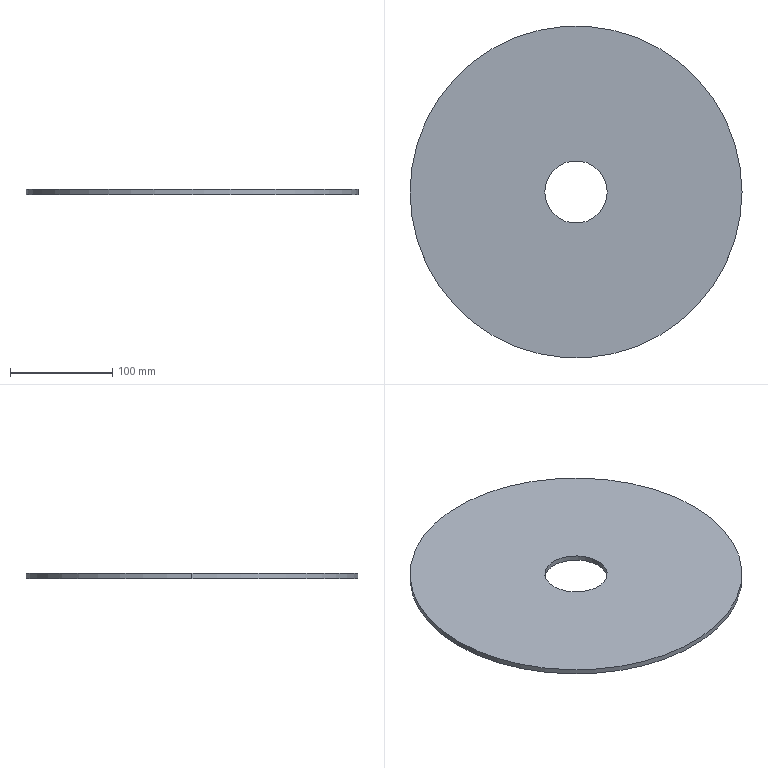Part | SolidWorks | features Extrusion 1 | 1 solid | 6 faces | box 325 x 325 x 5 mm | volume 400176 mm3 | cylinder 4 | plane 2 | commonest cylinder face diameters 61 x2 325 x2
STEP:
#1=CARTESIAN_POINT('',(-30.5,0.,5.));
#2=VERTEX_POINT('',#1);
#3=CARTESIAN_POINT('',(30.5,0.,5.));
#4=VERTEX_POINT('',#3);
#5=CARTESIAN_POINT('',(0.,0.,5.));
#6=DIRECTION('',(0.,0.,1.));
#7=DIRECTION('',(1.,0.,0.));
#8=AXIS2_PLACEMENT_3D('',#5,#6,#7);
#9=CIRCLE('',#8,30.5);
#10=EDGE_CURVE('',#2,#4,#9,.T.);
#11=ORIENTED_EDGE('',*,*,#10,.T.);
#12=CARTESIAN_POINT('',(30.5,0.,0.));
#13=VERTEX_POINT('',#12);
#14=CARTESIAN_POINT('',(30.5,0.,5.));
#15=DIRECTION('',(0.,0.,-1.));
#16=VECTOR('',#15,1000.);
#17=LINE('',#14,#16);
#18=EDGE_CURVE('',#4,#13,#17,.T.);
#19=ORIENTED_EDGE('',*,*,#18,.T.);
#20=CARTESIAN_POINT('',(-30.5,0.,0.));
#21=VERTEX_POINT('',#20);
#22=CARTESIAN_POINT('',(0.,0.,0.));
#23=DIRECTION('',(0.,0.,1.));
#24=DIRECTION('',(1.,0.,0.));
#25=AXIS2_PLACEMENT_3D('',#22,#23,#24);
#26=CIRCLE('',#25,30.5);
#27=EDGE_CURVE('',#21,#13,#26,.T.);
#28=ORIENTED_EDGE('',*,*,#27,.F.);
#29=CARTESIAN_POINT('',(-30.5,0.,5.));
#30=DIRECTION('',(0.,0.,-1.));
#31=VECTOR('',#30,1000.);
#32=LINE('',#29,#31);
#33=EDGE_CURVE('',#2,#21,#32,.T.);
#34=ORIENTED_EDGE('',*,*,#33,.F.);
#35=EDGE_LOOP('',(#11,#19,#28,#34));
#36=FACE_OUTER_BOUND('',#35,.T.);
#37=CARTESIAN_POINT('',(0.,0.,5.));
#38=DIRECTION('',(0.,0.,-1.));
#39=DIRECTION('',(-1.,0.,0.));
#40=AXIS2_PLACEMENT_3D('',#37,#38,#39);
#41=CYLINDRICAL_SURFACE('',#40,30.5);
#42=ADVANCED_FACE('',(#36),#41,.F.);
#43=CARTESIAN_POINT('',(162.5,0.,5.));
#44=VERTEX_POINT('',#43);
#45=CARTESIAN_POINT('',(-162.5,0.,5.));
#46=VERTEX_POINT('',#45);
#47=CARTESIAN_POINT('',(0.,0.,5.));
#48=DIRECTION('',(0.,0.,1.));
#49=DIRECTION('',(1.,0.,0.));
#50=AXIS2_PLACEMENT_3D('',#47,#48,#49);
#51=CIRCLE('',#50,162.5);
#52=EDGE_CURVE('',#44,#46,#51,.T.);
#53=ORIENTED_EDGE('',*,*,#52,.F.);
#54=CARTESIAN_POINT('',(162.5,0.,0.));
#55=VERTEX_POINT('',#54);
#56=CARTESIAN_POINT('',(162.5,0.,5.));
#57=DIRECTION('',(0.,0.,-1.));
#58=VECTOR('',#57,1000.);
#59=LINE('',#56,#58);
#60=EDGE_CURVE('',#44,#55,#59,.T.);
#61=ORIENTED_EDGE('',*,*,#60,.T.);
#62=CARTESIAN_POINT('',(-162.5,0.,0.));
#63=VERTEX_POINT('',#62);
#64=CARTESIAN_POINT('',(0.,0.,0.));
#65=DIRECTION('',(0.,0.,1.));
#66=DIRECTION('',(1.,0.,0.));
#67=AXIS2_PLACEMENT_3D('',#64,#65,#66);
#68=CIRCLE('',#67,162.5);
#69=EDGE_CURVE('',#55,#63,#68,.T.);
#70=ORIENTED_EDGE('',*,*,#69,.T.);
#71=CARTESIAN_POINT('',(-162.5,0.,5.));
#72=DIRECTION('',(0.,0.,-1.));
#73=VECTOR('',#72,1000.);
#74=LINE('',#71,#73);
#75=EDGE_CURVE('',#46,#63,#74,.T.);
#76=ORIENTED_EDGE('',*,*,#75,.F.);
#77=EDGE_LOOP('',(#53,#61,#70,#76));
#78=FACE_OUTER_BOUND('',#77,.T.);
#79=CARTESIAN_POINT('',(0.,0.,5.));
#80=DIRECTION('',(0.,0.,-1.));
#81=DIRECTION('',(-1.,0.,0.));
#82=AXIS2_PLACEMENT_3D('',#79,#80,#81);
#83=CYLINDRICAL_SURFACE('',#82,162.5);
#84=ADVANCED_FACE('',(#78),#83,.T.);
#85=CARTESIAN_POINT('',(0.,0.,5.));
#86=DIRECTION('',(0.,0.,1.));
#87=DIRECTION('',(1.,0.,0.));
#88=AXIS2_PLACEMENT_3D('',#85,#86,#87);
#89=CIRCLE('',#88,162.5);
#90=EDGE_CURVE('',#46,#44,#89,.T.);
#91=ORIENTED_EDGE('',*,*,#90,.T.);
#92=ORIENTED_EDGE('',*,*,#52,.T.);
#93=EDGE_LOOP('',(#91,#92));
#94=FACE_OUTER_BOUND('',#93,.T.);
#95=ORIENTED_EDGE('',*,*,#10,.F.);
#96=CARTESIAN_POINT('',(0.,0.,5.));
#97=DIRECTION('',(0.,0.,1.));
#98=DIRECTION('',(1.,0.,0.));
#99=AXIS2_PLACEMENT_3D('',#96,#97,#98);
#100=CIRCLE('',#99,30.5);
#101=EDGE_CURVE('',#4,#2,#100,.T.);
#102=ORIENTED_EDGE('',*,*,#101,.F.);
#103=EDGE_LOOP('',(#95,#102));
#104=FACE_BOUND('',#103,.T.);
#105=CARTESIAN_POINT('',(0.,0.,5.));
#106=DIRECTION('',(0.,0.,1.));
#107=DIRECTION('',(1.,0.,0.));
#108=AXIS2_PLACEMENT_3D('',#105,#106,#107);
#109=PLANE('',#108);
#110=ADVANCED_FACE('',(#94,#104),#109,.T.);
#111=CARTESIAN_POINT('',(0.,0.,0.));
#112=DIRECTION('',(0.,0.,1.));
#113=DIRECTION('',(1.,0.,0.));
#114=AXIS2_PLACEMENT_3D('',#111,#112,#113);
#115=CIRCLE('',#114,162.5);
#116=EDGE_CURVE('',#63,#55,#115,.T.);
#117=ORIENTED_EDGE('',*,*,#116,.F.);
#118=ORIENTED_EDGE('',*,*,#69,.F.);
#119=EDGE_LOOP('',(#117,#118));
#120=FACE_OUTER_BOUND('',#119,.T.);
#121=ORIENTED_EDGE('',*,*,#27,.T.);
#122=CARTESIAN_POINT('',(0.,0.,0.));
#123=DIRECTION('',(0.,0.,1.));
#124=DIRECTION('',(1.,0.,0.));
#125=AXIS2_PLACEMENT_3D('',#122,#123,#124);
#126=CIRCLE('',#125,30.5);
#127=EDGE_CURVE('',#13,#21,#126,.T.);
#128=ORIENTED_EDGE('',*,*,#127,.T.);
#129=EDGE_LOOP('',(#121,#128));
#130=FACE_BOUND('',#129,.T.);
#131=CARTESIAN_POINT('',(0.,0.,0.));
#132=DIRECTION('',(0.,0.,1.));
#133=DIRECTION('',(1.,0.,0.));
#134=AXIS2_PLACEMENT_3D('',#131,#132,#133);
#135=PLANE('',#134);
#136=ADVANCED_FACE('',(#120,#130),#135,.F.);
#137=ORIENTED_EDGE('',*,*,#60,.F.);
#138=ORIENTED_EDGE('',*,*,#90,.F.);
#139=ORIENTED_EDGE('',*,*,#75,.T.);
#140=ORIENTED_EDGE('',*,*,#116,.T.);
#141=EDGE_LOOP('',(#137,#138,#139,#140));
#142=FACE_OUTER_BOUND('',#141,.T.);
#143=CARTESIAN_POINT('',(0.,0.,5.));
#144=DIRECTION('',(0.,0.,-1.));
#145=DIRECTION('',(-1.,0.,0.));
#146=AXIS2_PLACEMENT_3D('',#143,#144,#145);
#147=CYLINDRICAL_SURFACE('',#146,162.5);
#148=ADVANCED_FACE('',(#142),#147,.T.);
#149=ORIENTED_EDGE('',*,*,#18,.F.);
#150=ORIENTED_EDGE('',*,*,#101,.T.);
#151=ORIENTED_EDGE('',*,*,#33,.T.);
#152=ORIENTED_EDGE('',*,*,#127,.F.);
#153=EDGE_LOOP('',(#149,#150,#151,#152));
#154=FACE_OUTER_BOUND('',#153,.T.);
#155=CARTESIAN_POINT('',(0.,0.,5.));
#156=DIRECTION('',(0.,0.,-1.));
#157=DIRECTION('',(-1.,0.,0.));
#158=AXIS2_PLACEMENT_3D('',#155,#156,#157);
#159=CYLINDRICAL_SURFACE('',#158,30.5);
#160=ADVANCED_FACE('',(#154),#159,.F.);
#161=CLOSED_SHELL('',(#42,#84,#110,#136,#148,#160));
#162=MANIFOLD_SOLID_BREP('',#161);
#163=CARTESIAN_POINT('',(0.,0.,0.));
#164=DIRECTION('',(0.,0.,1.));
#165=DIRECTION('',(1.,0.,0.));
#166=AXIS2_PLACEMENT_3D('',#163,#164,#165);
#167=(LENGTH_UNIT()NAMED_UNIT(*)SI_UNIT(.MILLI.,.METRE.));
#168=UNCERTAINTY_MEASURE_WITH_UNIT(LENGTH_MEASURE(0.00001),#167,'','');
#169=(NAMED_UNIT(*)PLANE_ANGLE_UNIT()SI_UNIT($,.RADIAN.));
#170=(NAMED_UNIT(*)SI_UNIT($,.STERADIAN.)SOLID_ANGLE_UNIT());
#171=(GEOMETRIC_REPRESENTATION_CONTEXT(3)GLOBAL_UNCERTAINTY_ASSIGNED_CONTEXT((#168))GLOBAL_UNIT_ASSIGNED_CONTEXT((#167,#169,#170))REPRESENTATION_CONTEXT('',''));
#172=ADVANCED_BREP_SHAPE_REPRESENTATION('',(#162,#166),#171);